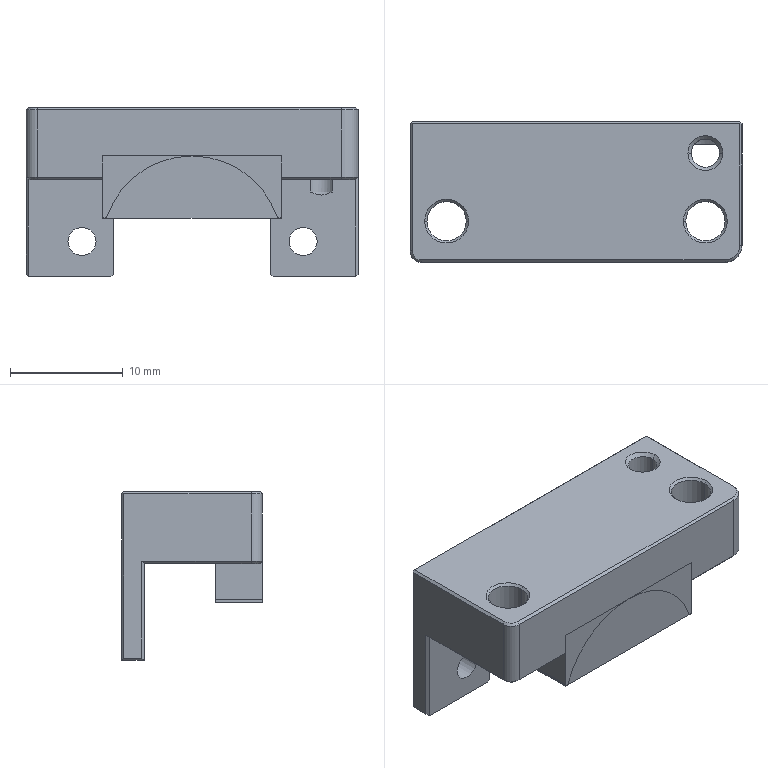NC program | NX | posted with a generic post | part box 29.5 x 12.5 x 15 mm
Whole program:
N10 G17 G21 G94 G90
(DRILLING_COPY_1_COPY_1 , TOOL : D6A45)
N12 T01 M6
N14 G54
N16 G17 G0 G90 X-9.875 Y-11.9 B0. C0. S5000 M3
N18 G43 Z30. H1
N20 G94 G81 G98 Z-1.45 F250. R3.
N22 X9.775
N24 G80
N26 G0 X9.775 Y-11.9 Z30.
N28 M5
(DRILLING_COPY_1_COPY_COPY_COPY , TOOL : 2.5ZT)
N30 T12 M6
N32 G54
N34 G17 G0 G90 X-9.875 Y-11.9 B0. C0. S2000 M3
N36 G43 Z30. H12
N38 G94 G83 G98 Z-4.251 F150. Q2. R3.
N40 X9.775
N42 G80
N44 G0 X9.775 Y-11.9 Z30.
N46 M5
N48 M2